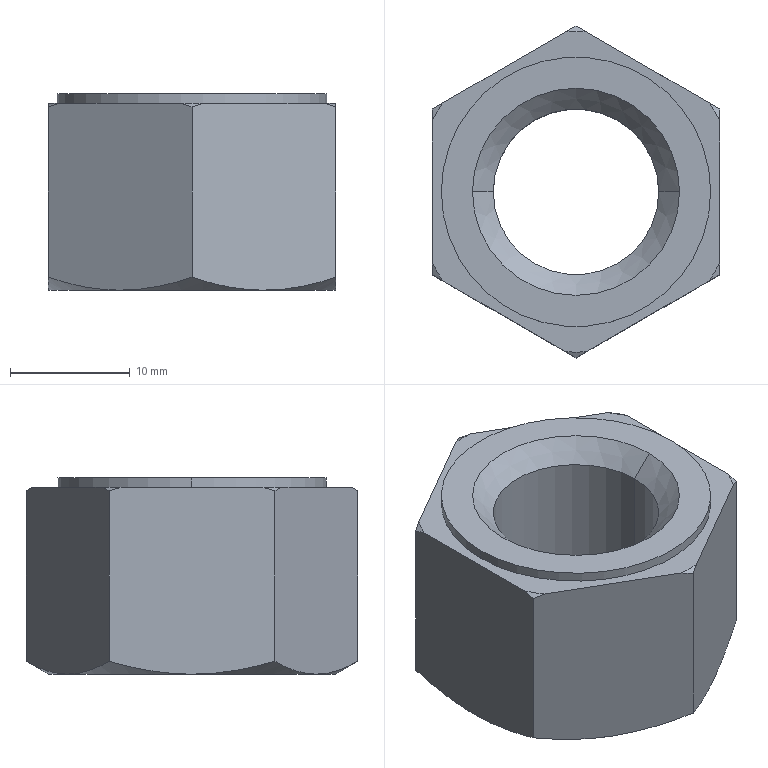Part | SolidWorks | features BaseBody 1 | 1 solid | 29 faces | box 24 x 27.713 x 16.4 mm | volume 5478 mm3 | cone 16 | plane 9 | cylinder 4 | commonest cylinder face diameters 13.835 x2 22.5 x2
STEP:
#1=CARTESIAN_POINT('',(11.25,0.,15.6));
#2=VERTEX_POINT('',#1);
#3=CARTESIAN_POINT('',(-11.25,0.,15.6));
#4=VERTEX_POINT('',#3);
#5=CARTESIAN_POINT('',(0.,0.,15.6));
#6=DIRECTION('',(0.,0.,1.));
#7=DIRECTION('',(1.,0.,0.));
#8=AXIS2_PLACEMENT_3D('',#5,#6,#7);
#9=CIRCLE('',#8,11.25);
#10=EDGE_CURVE('',#2,#4,#9,.T.);
#11=ORIENTED_EDGE('',*,*,#10,.T.);
#12=CARTESIAN_POINT('',(-11.25,0.,16.4));
#13=VERTEX_POINT('',#12);
#14=CARTESIAN_POINT('',(-11.25,0.,15.6));
#15=DIRECTION('',(0.,0.,1.));
#16=VECTOR('',#15,1000.);
#17=LINE('',#14,#16);
#18=EDGE_CURVE('',#4,#13,#17,.T.);
#19=ORIENTED_EDGE('',*,*,#18,.T.);
#20=CARTESIAN_POINT('',(11.25,0.,16.4));
#21=VERTEX_POINT('',#20);
#22=CARTESIAN_POINT('',(0.,0.,16.4));
#23=DIRECTION('',(0.,0.,1.));
#24=DIRECTION('',(1.,0.,0.));
#25=AXIS2_PLACEMENT_3D('',#22,#23,#24);
#26=CIRCLE('',#25,11.25);
#27=EDGE_CURVE('',#21,#13,#26,.T.);
#28=ORIENTED_EDGE('',*,*,#27,.F.);
#29=CARTESIAN_POINT('',(11.25,0.,15.6));
#30=DIRECTION('',(0.,0.,1.));
#31=VECTOR('',#30,1000.);
#32=LINE('',#29,#31);
#33=EDGE_CURVE('',#2,#21,#32,.T.);
#34=ORIENTED_EDGE('',*,*,#33,.F.);
#35=EDGE_LOOP('',(#11,#19,#28,#34));
#36=FACE_OUTER_BOUND('',#35,.T.);
#37=CARTESIAN_POINT('',(0.,0.,15.6));
#38=DIRECTION('',(0.,0.,1.));
#39=DIRECTION('',(1.,0.,0.));
#40=AXIS2_PLACEMENT_3D('',#37,#38,#39);
#41=CYLINDRICAL_SURFACE('',#40,11.25);
#42=ADVANCED_FACE('',(#36),#41,.T.);
#43=CARTESIAN_POINT('',(-6.918,0.,14.668));
#44=VERTEX_POINT('',#43);
#45=CARTESIAN_POINT('',(6.918,0.,14.668));
#46=VERTEX_POINT('',#45);
#47=CARTESIAN_POINT('',(0.,0.,14.668));
#48=DIRECTION('',(0.,0.,1.));
#49=DIRECTION('',(1.,0.,0.));
#50=AXIS2_PLACEMENT_3D('',#47,#48,#49);
#51=CIRCLE('',#50,6.918);
#52=EDGE_CURVE('',#44,#46,#51,.T.);
#53=ORIENTED_EDGE('',*,*,#52,.F.);
#54=CARTESIAN_POINT('',(-8.65,0.,16.4));
#55=VERTEX_POINT('',#54);
#56=CARTESIAN_POINT('',(-6.918,0.,14.668));
#57=DIRECTION('',(-0.7071,0.,0.7071));
#58=VECTOR('',#57,1000.);
#59=LINE('',#56,#58);
#60=EDGE_CURVE('',#44,#55,#59,.T.);
#61=ORIENTED_EDGE('',*,*,#60,.T.);
#62=CARTESIAN_POINT('',(8.65,0.,16.4));
#63=VERTEX_POINT('',#62);
#64=CARTESIAN_POINT('',(0.,0.,16.4));
#65=DIRECTION('',(0.,0.,-1.));
#66=DIRECTION('',(1.,0.,0.));
#67=AXIS2_PLACEMENT_3D('',#64,#65,#66);
#68=CIRCLE('',#67,8.65);
#69=EDGE_CURVE('',#63,#55,#68,.T.);
#70=ORIENTED_EDGE('',*,*,#69,.F.);
#71=CARTESIAN_POINT('',(6.918,0.,14.668));
#72=DIRECTION('',(0.7071,0.,0.7071));
#73=VECTOR('',#72,1000.);
#74=LINE('',#71,#73);
#75=EDGE_CURVE('',#46,#63,#74,.T.);
#76=ORIENTED_EDGE('',*,*,#75,.F.);
#77=EDGE_LOOP('',(#53,#61,#70,#76));
#78=FACE_OUTER_BOUND('',#77,.T.);
#79=CARTESIAN_POINT('',(0.,0.,14.668));
#80=DIRECTION('',(0.,0.,1.));
#81=DIRECTION('',(1.,0.,0.));
#82=AXIS2_PLACEMENT_3D('',#79,#80,#81);
#83=CONICAL_SURFACE('',#82,6.918,0.7854);
#84=ADVANCED_FACE('',(#78),#83,.F.);
#85=CARTESIAN_POINT('',(6.918,0.,1.733));
#86=VERTEX_POINT('',#85);
#87=CARTESIAN_POINT('',(-6.918,0.,1.733));
#88=VERTEX_POINT('',#87);
#89=CARTESIAN_POINT('',(0.,0.,1.733));
#90=DIRECTION('',(0.,0.,-1.));
#91=DIRECTION('',(1.,0.,0.));
#92=AXIS2_PLACEMENT_3D('',#89,#90,#91);
#93=CIRCLE('',#92,6.918);
#94=EDGE_CURVE('',#86,#88,#93,.T.);
#95=ORIENTED_EDGE('',*,*,#94,.F.);
#96=CARTESIAN_POINT('',(8.65,0.,0.));
#97=VERTEX_POINT('',#96);
#98=CARTESIAN_POINT('',(8.65,0.,0.));
#99=DIRECTION('',(0.7071,0.,-0.7071));
#100=VECTOR('',#99,1000.);
#101=LINE('',#98,#100);
#102=EDGE_CURVE('',#86,#97,#101,.T.);
#103=ORIENTED_EDGE('',*,*,#102,.T.);
#104=CARTESIAN_POINT('',(-8.65,0.,0.));
#105=VERTEX_POINT('',#104);
#106=CARTESIAN_POINT('',(0.,0.,0.));
#107=DIRECTION('',(0.,0.,1.));
#108=DIRECTION('',(1.,0.,0.));
#109=AXIS2_PLACEMENT_3D('',#106,#107,#108);
#110=CIRCLE('',#109,8.65);
#111=EDGE_CURVE('',#105,#97,#110,.T.);
#112=ORIENTED_EDGE('',*,*,#111,.F.);
#113=CARTESIAN_POINT('',(-8.65,0.,0.));
#114=DIRECTION('',(-0.7071,0.,-0.7071));
#115=VECTOR('',#114,1000.);
#116=LINE('',#113,#115);
#117=EDGE_CURVE('',#88,#105,#116,.T.);
#118=ORIENTED_EDGE('',*,*,#117,.F.);
#119=EDGE_LOOP('',(#95,#103,#112,#118));
#120=FACE_OUTER_BOUND('',#119,.T.);
#121=CARTESIAN_POINT('',(0.,0.,0.));
#122=DIRECTION('',(0.,0.,-1.));
#123=DIRECTION('',(-1.,0.,0.));
#124=AXIS2_PLACEMENT_3D('',#121,#122,#123);
#125=CONICAL_SURFACE('',#124,8.65,0.7854);
#126=ADVANCED_FACE('',(#120),#125,.F.);
#127=ORIENTED_EDGE('',*,*,#52,.T.);
#128=CARTESIAN_POINT('',(6.918,0.,16.4));
#129=DIRECTION('',(0.,0.,-1.));
#130=VECTOR('',#129,1000.);
#131=LINE('',#128,#130);
#132=EDGE_CURVE('',#46,#86,#131,.T.);
#133=ORIENTED_EDGE('',*,*,#132,.T.);
#134=ORIENTED_EDGE('',*,*,#94,.T.);
#135=CARTESIAN_POINT('',(-6.918,0.,16.4));
#136=DIRECTION('',(0.,0.,-1.));
#137=VECTOR('',#136,1000.);
#138=LINE('',#135,#137);
#139=EDGE_CURVE('',#44,#88,#138,.T.);
#140=ORIENTED_EDGE('',*,*,#139,.F.);
#141=EDGE_LOOP('',(#127,#133,#134,#140));
#142=FACE_OUTER_BOUND('',#141,.T.);
#143=CARTESIAN_POINT('',(0.,0.,16.4));
#144=DIRECTION('',(0.,0.,-1.));
#145=DIRECTION('',(-1.,0.,0.));
#146=AXIS2_PLACEMENT_3D('',#143,#144,#145);
#147=CYLINDRICAL_SURFACE('',#146,6.918);
#148=ADVANCED_FACE('',(#142),#147,.F.);
#149=CARTESIAN_POINT('',(11.136,7.427,15.6));
#150=VERTEX_POINT('',#149);
#151=CARTESIAN_POINT('',(0.8637,13.358,15.6));
#152=VERTEX_POINT('',#151);
#153=CARTESIAN_POINT('',(12.,6.928,15.6));
#154=DIRECTION('',(-0.866,0.5,0.));
#155=VECTOR('',#154,1000.);
#156=LINE('',#153,#155);
#157=EDGE_CURVE('',#150,#152,#156,.T.);
#158=ORIENTED_EDGE('',*,*,#157,.F.);
#159=CARTESIAN_POINT('',(12.,6.928,15.328));
#160=VERTEX_POINT('',#159);
#161=CARTESIAN_POINT('',(12.,6.928,15.328));
#162=CARTESIAN_POINT('',(11.713,7.094,15.424));
#163=CARTESIAN_POINT('',(11.425,7.26,15.515));
#164=CARTESIAN_POINT('',(11.136,7.427,15.6));
#165=B_SPLINE_CURVE_WITH_KNOTS('',3,(#161,#162,#163,#164),.UNSPECIFIED.,.F.,.F.,(4,4),(0.000000238,0.001026),.UNSPECIFIED.);
#166=EDGE_CURVE('',#160,#150,#165,.T.);
#167=ORIENTED_EDGE('',*,*,#166,.F.);
#168=CARTESIAN_POINT('',(12.,6.928,1.072));
#169=VERTEX_POINT('',#168);
#170=CARTESIAN_POINT('',(12.,6.928,16.4));
#171=DIRECTION('',(0.,0.,-1.));
#172=VECTOR('',#171,1000.);
#173=LINE('',#170,#172);
#174=EDGE_CURVE('',#160,#169,#173,.T.);
#175=ORIENTED_EDGE('',*,*,#174,.T.);
#176=CARTESIAN_POINT('',(6.,10.392,0.));
#177=VERTEX_POINT('',#176);
#178=CARTESIAN_POINT('',(6.,10.392,0.));
#179=CARTESIAN_POINT('',(6.509,10.098,0.));
#180=CARTESIAN_POINT('',(7.021,9.803,0.02533));
#181=CARTESIAN_POINT('',(8.033,9.219,0.1234));
#182=CARTESIAN_POINT('',(8.535,8.929,0.196));
#183=CARTESIAN_POINT('',(10.034,8.063,0.476));
#184=CARTESIAN_POINT('',(11.021,7.493,0.7454));
#185=CARTESIAN_POINT('',(12.,6.928,1.072));
#186=B_SPLINE_CURVE_WITH_KNOTS('',3,(#178,#179,#180,#181,#182,#183,#184,#185),.UNSPECIFIED.,.F.,.F.,(4,2,2,4),(0.00701,0.008756,0.0105,0.01399),.UNSPECIFIED.);
#187=EDGE_CURVE('',#177,#169,#186,.T.);
#188=ORIENTED_EDGE('',*,*,#187,.F.);
#189=CARTESIAN_POINT('',(0.,13.856,1.072));
#190=VERTEX_POINT('',#189);
#191=CARTESIAN_POINT('',(0.,13.856,1.072));
#192=CARTESIAN_POINT('',(0.9815,13.29,0.7446));
#193=CARTESIAN_POINT('',(1.97,12.719,0.4751));
#194=CARTESIAN_POINT('',(3.968,11.565,0.1021));
#195=CARTESIAN_POINT('',(4.978,10.982,0.));
#196=CARTESIAN_POINT('',(6.,10.392,0.));
#197=B_SPLINE_CURVE_WITH_KNOTS('',3,(#191,#192,#193,#194,#195,#196),.UNSPECIFIED.,.F.,.F.,(4,2,4),(0.000000238,0.003505,0.00701),.UNSPECIFIED.);
#198=EDGE_CURVE('',#190,#177,#197,.T.);
#199=ORIENTED_EDGE('',*,*,#198,.F.);
#200=CARTESIAN_POINT('',(0.,13.856,15.328));
#201=VERTEX_POINT('',#200);
#202=CARTESIAN_POINT('',(0.,13.856,16.4));
#203=DIRECTION('',(0.,0.,-1.));
#204=VECTOR('',#203,1000.);
#205=LINE('',#202,#204);
#206=EDGE_CURVE('',#201,#190,#205,.T.);
#207=ORIENTED_EDGE('',*,*,#206,.F.);
#208=CARTESIAN_POINT('',(0.8637,13.358,15.6));
#209=CARTESIAN_POINT('',(0.575,13.524,15.515));
#210=CARTESIAN_POINT('',(0.2872,13.691,15.424));
#211=CARTESIAN_POINT('',(0.,13.856,15.328));
#212=B_SPLINE_CURVE_WITH_KNOTS('',3,(#208,#209,#210,#211),.UNSPECIFIED.,.F.,.F.,(4,4),(0.01297,0.01399),.UNSPECIFIED.);
#213=EDGE_CURVE('',#152,#201,#212,.T.);
#214=ORIENTED_EDGE('',*,*,#213,.F.);
#215=EDGE_LOOP('',(#158,#167,#175,#188,#199,#207,#214));
#216=FACE_OUTER_BOUND('',#215,.T.);
#217=CARTESIAN_POINT('',(12.,6.928,16.4));
#218=DIRECTION('',(-0.5,-0.866,0.));
#219=DIRECTION('',(0.866,-0.5,0.));
#220=AXIS2_PLACEMENT_3D('',#217,#218,#219);
#221=PLANE('',#220);
#222=ADVANCED_FACE('',(#216),#221,.F.);
#223=CARTESIAN_POINT('',(-0.8637,13.358,15.6));
#224=VERTEX_POINT('',#223);
#225=CARTESIAN_POINT('',(-11.136,7.427,15.6));
#226=VERTEX_POINT('',#225);
#227=CARTESIAN_POINT('',(0.,13.856,15.6));
#228=DIRECTION('',(-0.866,-0.5,0.));
#229=VECTOR('',#228,1000.);
#230=LINE('',#227,#229);
#231=EDGE_CURVE('',#224,#226,#230,.T.);
#232=ORIENTED_EDGE('',*,*,#231,.F.);
#233=CARTESIAN_POINT('',(0.,13.856,15.328));
#234=CARTESIAN_POINT('',(-0.2873,13.691,15.424));
#235=CARTESIAN_POINT('',(-0.5751,13.524,15.515));
#236=CARTESIAN_POINT('',(-0.8637,13.358,15.6));
#237=B_SPLINE_CURVE_WITH_KNOTS('',3,(#233,#234,#235,#236),.UNSPECIFIED.,.F.,.F.,(4,4),(0.000000238,0.001026),.UNSPECIFIED.);
#238=EDGE_CURVE('',#201,#224,#237,.T.);
#239=ORIENTED_EDGE('',*,*,#238,.F.);
#240=ORIENTED_EDGE('',*,*,#206,.T.);
#241=CARTESIAN_POINT('',(-6.,10.392,0.));
#242=VERTEX_POINT('',#241);
#243=CARTESIAN_POINT('',(-6.,10.392,0.));
#244=CARTESIAN_POINT('',(-5.491,10.686,0.));
#245=CARTESIAN_POINT('',(-4.979,10.982,0.02533));
#246=CARTESIAN_POINT('',(-3.967,11.566,0.1234));
#247=CARTESIAN_POINT('',(-3.465,11.856,0.196));
#248=CARTESIAN_POINT('',(-1.966,12.721,0.476));
#249=CARTESIAN_POINT('',(-0.9791,13.291,0.7454));
#250=CARTESIAN_POINT('',(0.,13.856,1.072));
#251=B_SPLINE_CURVE_WITH_KNOTS('',3,(#243,#244,#245,#246,#247,#248,#249,#250),.UNSPECIFIED.,.F.,.F.,(4,2,2,4),(0.00701,0.008756,0.0105,0.01399),.UNSPECIFIED.);
#252=EDGE_CURVE('',#242,#190,#251,.T.);
#253=ORIENTED_EDGE('',*,*,#252,.F.);
#254=CARTESIAN_POINT('',(-12.,6.928,1.072));
#255=VERTEX_POINT('',#254);
#256=CARTESIAN_POINT('',(-12.,6.928,1.072));
#257=CARTESIAN_POINT('',(-11.018,7.495,0.7446));
#258=CARTESIAN_POINT('',(-10.03,8.066,0.4751));
#259=CARTESIAN_POINT('',(-8.032,9.219,0.1021));
#260=CARTESIAN_POINT('',(-7.022,9.802,0.));
#261=CARTESIAN_POINT('',(-6.,10.392,0.));
#262=B_SPLINE_CURVE_WITH_KNOTS('',3,(#256,#257,#258,#259,#260,#261),.UNSPECIFIED.,.F.,.F.,(4,2,4),(0.000000238,0.003505,0.00701),.UNSPECIFIED.);
#263=EDGE_CURVE('',#255,#242,#262,.T.);
#264=ORIENTED_EDGE('',*,*,#263,.F.);
#265=CARTESIAN_POINT('',(-12.,6.928,15.328));
#266=VERTEX_POINT('',#265);
#267=CARTESIAN_POINT('',(-12.,6.928,16.4));
#268=DIRECTION('',(0.,0.,-1.));
#269=VECTOR('',#268,1000.);
#270=LINE('',#267,#269);
#271=EDGE_CURVE('',#266,#255,#270,.T.);
#272=ORIENTED_EDGE('',*,*,#271,.F.);
#273=CARTESIAN_POINT('',(-11.136,7.427,15.6));
#274=CARTESIAN_POINT('',(-11.425,7.26,15.515));
#275=CARTESIAN_POINT('',(-11.713,7.094,15.424));
#276=CARTESIAN_POINT('',(-12.,6.928,15.328));
#277=B_SPLINE_CURVE_WITH_KNOTS('',3,(#273,#274,#275,#276),.UNSPECIFIED.,.F.,.F.,(4,4),(0.01297,0.01399),.UNSPECIFIED.);
#278=EDGE_CURVE('',#226,#266,#277,.T.);
#279=ORIENTED_EDGE('',*,*,#278,.F.);
#280=EDGE_LOOP('',(#232,#239,#240,#253,#264,#272,#279));
#281=FACE_OUTER_BOUND('',#280,.T.);
#282=CARTESIAN_POINT('',(0.,13.856,16.4));
#283=DIRECTION('',(0.5,-0.866,0.));
#284=DIRECTION('',(0.866,0.5,0.));
#285=AXIS2_PLACEMENT_3D('',#282,#283,#284);
#286=PLANE('',#285);
#287=ADVANCED_FACE('',(#281),#286,.F.);
#288=CARTESIAN_POINT('',(-12.,5.931,15.6));
#289=VERTEX_POINT('',#288);
#290=CARTESIAN_POINT('',(-12.,-5.931,15.6));
#291=VERTEX_POINT('',#290);
#292=CARTESIAN_POINT('',(-12.,6.928,15.6));
#293=DIRECTION('',(0.,-1.,0.));
#294=VECTOR('',#293,1000.);
#295=LINE('',#292,#294);
#296=EDGE_CURVE('',#289,#291,#295,.T.);
#297=ORIENTED_EDGE('',*,*,#296,.F.);
#298=CARTESIAN_POINT('',(-12.,6.928,15.328));
#299=CARTESIAN_POINT('',(-12.,6.597,15.424));
#300=CARTESIAN_POINT('',(-12.,6.265,15.515));
#301=CARTESIAN_POINT('',(-12.,5.931,15.6));
#302=B_SPLINE_CURVE_WITH_KNOTS('',3,(#298,#299,#300,#301),.UNSPECIFIED.,.F.,.F.,(4,4),(0.04083,0.04186),.UNSPECIFIED.);
#303=EDGE_CURVE('',#266,#289,#302,.T.);
#304=ORIENTED_EDGE('',*,*,#303,.F.);
#305=ORIENTED_EDGE('',*,*,#271,.T.);
#306=CARTESIAN_POINT('',(-12.,0.,0.));
#307=VERTEX_POINT('',#306);
#308=CARTESIAN_POINT('',(-12.,0.,0.));
#309=CARTESIAN_POINT('',(-12.,0.5864,0.));
#310=CARTESIAN_POINT('',(-12.,1.176,0.02502));
#311=CARTESIAN_POINT('',(-12.,2.355,0.1241));
#312=CARTESIAN_POINT('',(-12.,2.939,0.1975));
#313=CARTESIAN_POINT('',(-12.,4.673,0.4791));
#314=CARTESIAN_POINT('',(-12.,5.808,0.7483));
#315=CARTESIAN_POINT('',(-12.,6.928,1.072));
#316=B_SPLINE_CURVE_WITH_KNOTS('',3,(#308,#309,#310,#311,#312,#313,#314,#315),.UNSPECIFIED.,.F.,.F.,(4,2,2,4),(0.01976,0.02151,0.02327,0.02678),.UNSPECIFIED.);
#317=EDGE_CURVE('',#307,#255,#316,.T.);
#318=ORIENTED_EDGE('',*,*,#317,.F.);
#319=CARTESIAN_POINT('',(-12.,-6.928,1.072));
#320=VERTEX_POINT('',#319);
#321=CARTESIAN_POINT('',(-12.,-6.928,1.072));
#322=CARTESIAN_POINT('',(-12.,-5.8,0.7462));
#323=CARTESIAN_POINT('',(-12.,-4.647,0.4736));
#324=CARTESIAN_POINT('',(-12.,-2.335,0.1008));
#325=CARTESIAN_POINT('',(-12.,-1.172,0.));
#326=CARTESIAN_POINT('',(-12.,0.,0.));
#327=B_SPLINE_CURVE_WITH_KNOTS('',3,(#321,#322,#323,#324,#325,#326),.UNSPECIFIED.,.F.,.F.,(4,2,4),(0.01275,0.01625,0.01976),.UNSPECIFIED.);
#328=EDGE_CURVE('',#320,#307,#327,.T.);
#329=ORIENTED_EDGE('',*,*,#328,.F.);
#330=CARTESIAN_POINT('',(-12.,-6.928,15.328));
#331=VERTEX_POINT('',#330);
#332=CARTESIAN_POINT('',(-12.,-6.928,16.4));
#333=DIRECTION('',(0.,0.,-1.));
#334=VECTOR('',#333,1000.);
#335=LINE('',#332,#334);
#336=EDGE_CURVE('',#331,#320,#335,.T.);
#337=ORIENTED_EDGE('',*,*,#336,.F.);
#338=CARTESIAN_POINT('',(-12.,-5.931,15.6));
#339=CARTESIAN_POINT('',(-12.,-6.265,15.514));
#340=CARTESIAN_POINT('',(-12.,-6.598,15.424));
#341=CARTESIAN_POINT('',(-12.,-6.928,15.328));
#342=B_SPLINE_CURVE_WITH_KNOTS('',3,(#338,#339,#340,#341),.UNSPECIFIED.,.F.,.F.,(4,4),(0.05382,0.05485),.UNSPECIFIED.);
#343=EDGE_CURVE('',#291,#331,#342,.T.);
#344=ORIENTED_EDGE('',*,*,#343,.F.);
#345=EDGE_LOOP('',(#297,#304,#305,#318,#329,#337,#344));
#346=FACE_OUTER_BOUND('',#345,.T.);
#347=CARTESIAN_POINT('',(-12.,6.928,16.4));
#348=DIRECTION('',(1.,0.,0.));
#349=DIRECTION('',(0.,1.,0.));
#350=AXIS2_PLACEMENT_3D('',#347,#348,#349);
#351=PLANE('',#350);
#352=ADVANCED_FACE('',(#346),#351,.F.);
#353=CARTESIAN_POINT('',(-11.136,-7.427,15.6));
#354=VERTEX_POINT('',#353);
#355=CARTESIAN_POINT('',(-0.8637,-13.358,15.6));
#356=VERTEX_POINT('',#355);
#357=CARTESIAN_POINT('',(-12.,-6.928,15.6));
#358=DIRECTION('',(0.866,-0.5,0.));
#359=VECTOR('',#358,1000.);
#360=LINE('',#357,#359);
#361=EDGE_CURVE('',#354,#356,#360,.T.);
#362=ORIENTED_EDGE('',*,*,#361,.F.);
#363=CARTESIAN_POINT('',(-12.,-6.928,15.328));
#364=CARTESIAN_POINT('',(-11.713,-7.094,15.424));
#365=CARTESIAN_POINT('',(-11.425,-7.26,15.515));
#366=CARTESIAN_POINT('',(-11.136,-7.427,15.6));
#367=B_SPLINE_CURVE_WITH_KNOTS('',3,(#363,#364,#365,#366),.UNSPECIFIED.,.F.,.F.,(4,4),(0.000000238,0.001026),.UNSPECIFIED.);
#368=EDGE_CURVE('',#331,#354,#367,.T.);
#369=ORIENTED_EDGE('',*,*,#368,.F.);
#370=ORIENTED_EDGE('',*,*,#336,.T.);
#371=CARTESIAN_POINT('',(-6.,-10.392,0.));
#372=VERTEX_POINT('',#371);
#373=CARTESIAN_POINT('',(-6.,-10.392,0.));
#374=CARTESIAN_POINT('',(-6.509,-10.098,0.));
#375=CARTESIAN_POINT('',(-7.021,-9.803,0.02533));
#376=CARTESIAN_POINT('',(-8.033,-9.219,0.1234));
#377=CARTESIAN_POINT('',(-8.535,-8.929,0.196));
#378=CARTESIAN_POINT('',(-10.034,-8.063,0.476));
#379=CARTESIAN_POINT('',(-11.021,-7.493,0.7454));
#380=CARTESIAN_POINT('',(-12.,-6.928,1.072));
#381=B_SPLINE_CURVE_WITH_KNOTS('',3,(#373,#374,#375,#376,#377,#378,#379,#380),.UNSPECIFIED.,.F.,.F.,(4,2,2,4),(0.00701,0.008756,0.0105,0.01399),.UNSPECIFIED.);
#382=EDGE_CURVE('',#372,#320,#381,.T.);
#383=ORIENTED_EDGE('',*,*,#382,.F.);
#384=CARTESIAN_POINT('',(0.,-13.856,1.072));
#385=VERTEX_POINT('',#384);
#386=CARTESIAN_POINT('',(0.,-13.856,1.072));
#387=CARTESIAN_POINT('',(-0.9815,-13.29,0.7446));
#388=CARTESIAN_POINT('',(-1.97,-12.719,0.4751));
#389=CARTESIAN_POINT('',(-3.968,-11.565,0.1021));
#390=CARTESIAN_POINT('',(-4.978,-10.982,0.));
#391=CARTESIAN_POINT('',(-6.,-10.392,0.));
#392=B_SPLINE_CURVE_WITH_KNOTS('',3,(#386,#387,#388,#389,#390,#391),.UNSPECIFIED.,.F.,.F.,(4,2,4),(0.000000238,0.003505,0.00701),.UNSPECIFIED.);
#393=EDGE_CURVE('',#385,#372,#392,.T.);
#394=ORIENTED_EDGE('',*,*,#393,.F.);
#395=CARTESIAN_POINT('',(0.,-13.856,15.328));
#396=VERTEX_POINT('',#395);
#397=CARTESIAN_POINT('',(0.,-13.856,16.4));
#398=DIRECTION('',(0.,0.,-1.));
#399=VECTOR('',#398,1000.);
#400=LINE('',#397,#399);
#401=EDGE_CURVE('',#396,#385,#400,.T.);
#402=ORIENTED_EDGE('',*,*,#401,.F.);
#403=CARTESIAN_POINT('',(-0.8637,-13.358,15.6));
#404=CARTESIAN_POINT('',(-0.575,-13.524,15.515));
#405=CARTESIAN_POINT('',(-0.2872,-13.691,15.424));
#406=CARTESIAN_POINT('',(0.,-13.856,15.328));
#407=B_SPLINE_CURVE_WITH_KNOTS('',3,(#403,#404,#405,#406),.UNSPECIFIED.,.F.,.F.,(4,4),(0.01297,0.01399),.UNSPECIFIED.);
#408=EDGE_CURVE('',#356,#396,#407,.T.);
#409=ORIENTED_EDGE('',*,*,#408,.F.);
#410=EDGE_LOOP('',(#362,#369,#370,#383,#394,#402,#409));
#411=FACE_OUTER_BOUND('',#410,.T.);
#412=CARTESIAN_POINT('',(-12.,-6.928,16.4));
#413=DIRECTION('',(0.5,0.866,0.));
#414=DIRECTION('',(-0.866,0.5,0.));
#415=AXIS2_PLACEMENT_3D('',#412,#413,#414);
#416=PLANE('',#415);
#417=ADVANCED_FACE('',(#411),#416,.F.);
#418=CARTESIAN_POINT('',(0.8637,-13.358,15.6));
#419=VERTEX_POINT('',#418);
#420=CARTESIAN_POINT('',(11.136,-7.427,15.6));
#421=VERTEX_POINT('',#420);
#422=CARTESIAN_POINT('',(0.,-13.856,15.6));
#423=DIRECTION('',(0.866,0.5,0.));
#424=VECTOR('',#423,1000.);
#425=LINE('',#422,#424);
#426=EDGE_CURVE('',#419,#421,#425,.T.);
#427=ORIENTED_EDGE('',*,*,#426,.F.);
#428=CARTESIAN_POINT('',(0.,-13.856,15.328));
#429=CARTESIAN_POINT('',(0.2873,-13.691,15.424));
#430=CARTESIAN_POINT('',(0.5751,-13.524,15.515));
#431=CARTESIAN_POINT('',(0.8637,-13.358,15.6));
#432=B_SPLINE_CURVE_WITH_KNOTS('',3,(#428,#429,#430,#431),.UNSPECIFIED.,.F.,.F.,(4,4),(0.000000238,0.001026),.UNSPECIFIED.);
#433=EDGE_CURVE('',#396,#419,#432,.T.);
#434=ORIENTED_EDGE('',*,*,#433,.F.);
#435=ORIENTED_EDGE('',*,*,#401,.T.);
#436=CARTESIAN_POINT('',(6.,-10.392,0.));
#437=VERTEX_POINT('',#436);
#438=CARTESIAN_POINT('',(6.,-10.392,0.));
#439=CARTESIAN_POINT('',(5.491,-10.686,0.));
#440=CARTESIAN_POINT('',(4.979,-10.982,0.02533));
#441=CARTESIAN_POINT('',(3.967,-11.566,0.1234));
#442=CARTESIAN_POINT('',(3.465,-11.856,0.196));
#443=CARTESIAN_POINT('',(1.966,-12.721,0.476));
#444=CARTESIAN_POINT('',(0.9791,-13.291,0.7454));
#445=CARTESIAN_POINT('',(0.,-13.856,1.072));
#446=B_SPLINE_CURVE_WITH_KNOTS('',3,(#438,#439,#440,#441,#442,#443,#444,#445),.UNSPECIFIED.,.F.,.F.,(4,2,2,4),(0.00701,0.008756,0.0105,0.01399),.UNSPECIFIED.);
#447=EDGE_CURVE('',#437,#385,#446,.T.);
#448=ORIENTED_EDGE('',*,*,#447,.F.);
#449=CARTESIAN_POINT('',(12.,-6.928,1.072));
#450=VERTEX_POINT('',#449);
#451=CARTESIAN_POINT('',(12.,-6.928,1.072));
#452=CARTESIAN_POINT('',(11.018,-7.495,0.7446));
#453=CARTESIAN_POINT('',(10.03,-8.066,0.4751));
#454=CARTESIAN_POINT('',(8.032,-9.219,0.1021));
#455=CARTESIAN_POINT('',(7.022,-9.802,0.));
#456=CARTESIAN_POINT('',(6.,-10.392,0.));
#457=B_SPLINE_CURVE_WITH_KNOTS('',3,(#451,#452,#453,#454,#455,#456),.UNSPECIFIED.,.F.,.F.,(4,2,4),(0.000000238,0.003505,0.00701),.UNSPECIFIED.);
#458=EDGE_CURVE('',#450,#437,#457,.T.);
#459=ORIENTED_EDGE('',*,*,#458,.F.);
#460=CARTESIAN_POINT('',(12.,-6.928,15.328));
#461=VERTEX_POINT('',#460);
#462=CARTESIAN_POINT('',(12.,-6.928,16.4));
#463=DIRECTION('',(0.,0.,-1.));
#464=VECTOR('',#463,1000.);
#465=LINE('',#462,#464);
#466=EDGE_CURVE('',#461,#450,#465,.T.);
#467=ORIENTED_EDGE('',*,*,#466,.F.);
#468=CARTESIAN_POINT('',(11.136,-7.427,15.6));
#469=CARTESIAN_POINT('',(11.425,-7.26,15.515));
#470=CARTESIAN_POINT('',(11.713,-7.094,15.424));
#471=CARTESIAN_POINT('',(12.,-6.928,15.328));
#472=B_SPLINE_CURVE_WITH_KNOTS('',3,(#468,#469,#470,#471),.UNSPECIFIED.,.F.,.F.,(4,4),(0.01297,0.01399),.UNSPECIFIED.);
#473=EDGE_CURVE('',#421,#461,#472,.T.);
#474=ORIENTED_EDGE('',*,*,#473,.F.);
#475=EDGE_LOOP('',(#427,#434,#435,#448,#459,#467,#474));
#476=FACE_OUTER_BOUND('',#475,.T.);
#477=CARTESIAN_POINT('',(0.,-13.856,16.4));
#478=DIRECTION('',(-0.5,0.866,0.));
#479=DIRECTION('',(-0.866,-0.5,0.));
#480=AXIS2_PLACEMENT_3D('',#477,#478,#479);
#481=PLANE('',#480);
#482=ADVANCED_FACE('',(#476),#481,.F.);
#483=CARTESIAN_POINT('',(12.,-5.931,15.6));
#484=VERTEX_POINT('',#483);
#485=CARTESIAN_POINT('',(12.,5.931,15.6));
#486=VERTEX_POINT('',#485);
#487=CARTESIAN_POINT('',(12.,-6.928,15.6));
#488=DIRECTION('',(0.,1.,0.));
#489=VECTOR('',#488,1000.);
#490=LINE('',#487,#489);
#491=EDGE_CURVE('',#484,#486,#490,.T.);
#492=ORIENTED_EDGE('',*,*,#491,.F.);
#493=CARTESIAN_POINT('',(12.,-6.928,15.328));
#494=CARTESIAN_POINT('',(12.,-6.598,15.424));
#495=CARTESIAN_POINT('',(12.,-6.265,15.514));
#496=CARTESIAN_POINT('',(12.,-5.931,15.6));
#497=B_SPLINE_CURVE_WITH_KNOTS('',3,(#493,#494,#495,#496),.UNSPECIFIED.,.F.,.F.,(4,4),(0.01275,0.01377),.UNSPECIFIED.);
#498=EDGE_CURVE('',#461,#484,#497,.T.);
#499=ORIENTED_EDGE('',*,*,#498,.F.);
#500=ORIENTED_EDGE('',*,*,#466,.T.);
#501=CARTESIAN_POINT('',(12.,0.,0.));
#502=VERTEX_POINT('',#501);
#503=CARTESIAN_POINT('',(12.,0.,0.));
#504=CARTESIAN_POINT('',(12.,-1.172,0.));
#505=CARTESIAN_POINT('',(12.,-2.335,0.1008));
#506=CARTESIAN_POINT('',(12.,-4.647,0.4736));
#507=CARTESIAN_POINT('',(12.,-5.8,0.7462));
#508=CARTESIAN_POINT('',(12.,-6.928,1.072));
#509=B_SPLINE_CURVE_WITH_KNOTS('',3,(#503,#504,#505,#506,#507,#508),.UNSPECIFIED.,.F.,.F.,(4,2,4),(0.04784,0.05135,0.05485),.UNSPECIFIED.);
#510=EDGE_CURVE('',#502,#450,#509,.T.);
#511=ORIENTED_EDGE('',*,*,#510,.F.);
#512=CARTESIAN_POINT('',(12.,6.928,1.072));
#513=CARTESIAN_POINT('',(12.,5.808,0.7483));
#514=CARTESIAN_POINT('',(12.,4.673,0.4791));
#515=CARTESIAN_POINT('',(12.,2.939,0.1975));
#516=CARTESIAN_POINT('',(12.,2.355,0.1241));
#517=CARTESIAN_POINT('',(12.,1.176,0.02502));
#518=CARTESIAN_POINT('',(12.,0.5864,0.));
#519=CARTESIAN_POINT('',(12.,0.,0.));
#520=B_SPLINE_CURVE_WITH_KNOTS('',3,(#512,#513,#514,#515,#516,#517,#518,#519),.UNSPECIFIED.,.F.,.F.,(4,2,2,4),(0.04083,0.04433,0.04609,0.04784),.UNSPECIFIED.);
#521=EDGE_CURVE('',#169,#502,#520,.T.);
#522=ORIENTED_EDGE('',*,*,#521,.F.);
#523=ORIENTED_EDGE('',*,*,#174,.F.);
#524=CARTESIAN_POINT('',(12.,5.931,15.6));
#525=CARTESIAN_POINT('',(12.,6.265,15.515));
#526=CARTESIAN_POINT('',(12.,6.597,15.424));
#527=CARTESIAN_POINT('',(12.,6.928,15.328));
#528=B_SPLINE_CURVE_WITH_KNOTS('',3,(#524,#525,#526,#527),.UNSPECIFIED.,.F.,.F.,(4,4),(0.02574,0.02678),.UNSPECIFIED.);
#529=EDGE_CURVE('',#486,#160,#528,.T.);
#530=ORIENTED_EDGE('',*,*,#529,.F.);
#531=EDGE_LOOP('',(#492,#499,#500,#511,#522,#523,#530));
#532=FACE_OUTER_BOUND('',#531,.T.);
#533=CARTESIAN_POINT('',(12.,-6.928,16.4));
#534=DIRECTION('',(-1.,0.,0.));
#535=DIRECTION('',(0.,-1.,0.));
#536=AXIS2_PLACEMENT_3D('',#533,#534,#535);
#537=PLANE('',#536);
#538=ADVANCED_FACE('',(#532),#537,.F.);
#539=ORIENTED_EDGE('',*,*,#69,.T.);
#540=CARTESIAN_POINT('',(0.,0.,16.4));
#541=DIRECTION('',(0.,0.,-1.));
#542=DIRECTION('',(1.,0.,0.));
#543=AXIS2_PLACEMENT_3D('',#540,#541,#542);
#544=CIRCLE('',#543,8.65);
#545=EDGE_CURVE('',#55,#63,#544,.T.);
#546=ORIENTED_EDGE('',*,*,#545,.T.);
#547=EDGE_LOOP('',(#539,#546));
#548=FACE_BOUND('',#547,.T.);
#549=ORIENTED_EDGE('',*,*,#27,.T.);
#550=CARTESIAN_POINT('',(0.,0.,16.4));
#551=DIRECTION('',(0.,0.,1.));
#552=DIRECTION('',(1.,0.,0.));
#553=AXIS2_PLACEMENT_3D('',#550,#551,#552);
#554=CIRCLE('',#553,11.25);
#555=EDGE_CURVE('',#13,#21,#554,.T.);
#556=ORIENTED_EDGE('',*,*,#555,.T.);
#557=EDGE_LOOP('',(#549,#556));
#558=FACE_OUTER_BOUND('',#557,.T.);
#559=CARTESIAN_POINT('',(-12.,20.785,16.4));
#560=DIRECTION('',(0.,0.,1.));
#561=DIRECTION('',(1.,0.,0.));
#562=AXIS2_PLACEMENT_3D('',#559,#560,#561);
#563=PLANE('',#562);
#564=ADVANCED_FACE('',(#548,#558),#563,.T.);
#565=ORIENTED_EDGE('',*,*,#498,.T.);
#566=CARTESIAN_POINT('',(0.,0.,15.6));
#567=DIRECTION('',(0.,0.,-1.));
#568=DIRECTION('',(1.,0.,0.));
#569=AXIS2_PLACEMENT_3D('',#566,#567,#568);
#570=CIRCLE('',#569,13.386);
#571=EDGE_CURVE('',#484,#421,#570,.T.);
#572=ORIENTED_EDGE('',*,*,#571,.T.);
#573=ORIENTED_EDGE('',*,*,#473,.T.);
#574=EDGE_LOOP('',(#565,#572,#573));
#575=FACE_OUTER_BOUND('',#574,.T.);
#576=CARTESIAN_POINT('',(0.,0.,16.4));
#577=DIRECTION('',(0.,0.,-1.));
#578=DIRECTION('',(1.,0.,0.));
#579=AXIS2_PLACEMENT_3D('',#576,#577,#578);
#580=CONICAL_SURFACE('',#579,12.,1.047);
#581=ADVANCED_FACE('',(#575),#580,.T.);
#582=ORIENTED_EDGE('',*,*,#433,.T.);
#583=CARTESIAN_POINT('',(0.,0.,15.6));
#584=DIRECTION('',(0.,0.,-1.));
#585=DIRECTION('',(1.,0.,0.));
#586=AXIS2_PLACEMENT_3D('',#583,#584,#585);
#587=CIRCLE('',#586,13.386);
#588=EDGE_CURVE('',#419,#356,#587,.T.);
#589=ORIENTED_EDGE('',*,*,#588,.T.);
#590=ORIENTED_EDGE('',*,*,#408,.T.);
#591=EDGE_LOOP('',(#582,#589,#590));
#592=FACE_OUTER_BOUND('',#591,.T.);
#593=CARTESIAN_POINT('',(0.,0.,16.4));
#594=DIRECTION('',(0.,0.,-1.));
#595=DIRECTION('',(1.,0.,0.));
#596=AXIS2_PLACEMENT_3D('',#593,#594,#595);
#597=CONICAL_SURFACE('',#596,12.,1.047);
#598=ADVANCED_FACE('',(#592),#597,.T.);
#599=ORIENTED_EDGE('',*,*,#368,.T.);
#600=CARTESIAN_POINT('',(0.,0.,15.6));
#601=DIRECTION('',(0.,0.,-1.));
#602=DIRECTION('',(1.,0.,0.));
#603=AXIS2_PLACEMENT_3D('',#600,#601,#602);
#604=CIRCLE('',#603,13.386);
#605=EDGE_CURVE('',#354,#291,#604,.T.);
#606=ORIENTED_EDGE('',*,*,#605,.T.);
#607=ORIENTED_EDGE('',*,*,#343,.T.);
#608=EDGE_LOOP('',(#599,#606,#607));
#609=FACE_OUTER_BOUND('',#608,.T.);
#610=CARTESIAN_POINT('',(0.,0.,16.4));
#611=DIRECTION('',(0.,0.,-1.));
#612=DIRECTION('',(1.,0.,0.));
#613=AXIS2_PLACEMENT_3D('',#610,#611,#612);
#614=CONICAL_SURFACE('',#613,12.,1.047);
#615=ADVANCED_FACE('',(#609),#614,.T.);
#616=ORIENTED_EDGE('',*,*,#303,.T.);
#617=CARTESIAN_POINT('',(0.,0.,15.6));
#618=DIRECTION('',(0.,0.,-1.));
#619=DIRECTION('',(1.,0.,0.));
#620=AXIS2_PLACEMENT_3D('',#617,#618,#619);
#621=CIRCLE('',#620,13.386);
#622=EDGE_CURVE('',#289,#226,#621,.T.);
#623=ORIENTED_EDGE('',*,*,#622,.T.);
#624=ORIENTED_EDGE('',*,*,#278,.T.);
#625=EDGE_LOOP('',(#616,#623,#624));
#626=FACE_OUTER_BOUND('',#625,.T.);
#627=CARTESIAN_POINT('',(0.,0.,16.4));
#628=DIRECTION('',(0.,0.,-1.));
#629=DIRECTION('',(1.,0.,0.));
#630=AXIS2_PLACEMENT_3D('',#627,#628,#629);
#631=CONICAL_SURFACE('',#630,12.,1.047);
#632=ADVANCED_FACE('',(#626),#631,.T.);
#633=ORIENTED_EDGE('',*,*,#238,.T.);
#634=CARTESIAN_POINT('',(0.,0.,15.6));
#635=DIRECTION('',(0.,0.,-1.));
#636=DIRECTION('',(1.,0.,0.));
#637=AXIS2_PLACEMENT_3D('',#634,#635,#636);
#638=CIRCLE('',#637,13.386);
#639=EDGE_CURVE('',#224,#152,#638,.T.);
#640=ORIENTED_EDGE('',*,*,#639,.T.);
#641=ORIENTED_EDGE('',*,*,#213,.T.);
#642=EDGE_LOOP('',(#633,#640,#641));
#643=FACE_OUTER_BOUND('',#642,.T.);
#644=CARTESIAN_POINT('',(0.,0.,16.4));
#645=DIRECTION('',(0.,0.,-1.));
#646=DIRECTION('',(1.,0.,0.));
#647=AXIS2_PLACEMENT_3D('',#644,#645,#646);
#648=CONICAL_SURFACE('',#647,12.,1.047);
#649=ADVANCED_FACE('',(#643),#648,.T.);
#650=ORIENTED_EDGE('',*,*,#166,.T.);
#651=CARTESIAN_POINT('',(0.,0.,15.6));
#652=DIRECTION('',(0.,0.,-1.));
#653=DIRECTION('',(1.,0.,0.));
#654=AXIS2_PLACEMENT_3D('',#651,#652,#653);
#655=CIRCLE('',#654,13.386);
#656=EDGE_CURVE('',#150,#486,#655,.T.);
#657=ORIENTED_EDGE('',*,*,#656,.T.);
#658=ORIENTED_EDGE('',*,*,#529,.T.);
#659=EDGE_LOOP('',(#650,#657,#658));
#660=FACE_OUTER_BOUND('',#659,.T.);
#661=CARTESIAN_POINT('',(0.,0.,16.4));
#662=DIRECTION('',(0.,0.,-1.));
#663=DIRECTION('',(1.,0.,0.));
#664=AXIS2_PLACEMENT_3D('',#661,#662,#663);
#665=CONICAL_SURFACE('',#664,12.,1.047);
#666=ADVANCED_FACE('',(#660),#665,.T.);
#667=ORIENTED_EDGE('',*,*,#111,.T.);
#668=CARTESIAN_POINT('',(0.,0.,0.));
#669=DIRECTION('',(0.,0.,1.));
#670=DIRECTION('',(1.,0.,0.));
#671=AXIS2_PLACEMENT_3D('',#668,#669,#670);
#672=CIRCLE('',#671,8.65);
#673=EDGE_CURVE('',#97,#105,#672,.T.);
#674=ORIENTED_EDGE('',*,*,#673,.T.);
#675=EDGE_LOOP('',(#667,#674));
#676=FACE_BOUND('',#675,.T.);
#677=CARTESIAN_POINT('',(0.,0.,0.));
#678=DIRECTION('',(0.,0.,-1.));
#679=DIRECTION('',(-1.,0.,0.));
#680=AXIS2_PLACEMENT_3D('',#677,#678,#679);
#681=CIRCLE('',#680,12.);
#682=EDGE_CURVE('',#177,#502,#681,.T.);
#683=ORIENTED_EDGE('',*,*,#682,.T.);
#684=CARTESIAN_POINT('',(0.,0.,0.));
#685=DIRECTION('',(0.,0.,-1.));
#686=DIRECTION('',(-1.,0.,0.));
#687=AXIS2_PLACEMENT_3D('',#684,#685,#686);
#688=CIRCLE('',#687,12.);
#689=EDGE_CURVE('',#502,#437,#688,.T.);
#690=ORIENTED_EDGE('',*,*,#689,.T.);
#691=CARTESIAN_POINT('',(0.,0.,0.));
#692=DIRECTION('',(0.,0.,-1.));
#693=DIRECTION('',(-1.,0.,0.));
#694=AXIS2_PLACEMENT_3D('',#691,#692,#693);
#695=CIRCLE('',#694,12.);
#696=EDGE_CURVE('',#437,#372,#695,.T.);
#697=ORIENTED_EDGE('',*,*,#696,.T.);
#698=CARTESIAN_POINT('',(0.,0.,0.));
#699=DIRECTION('',(0.,0.,-1.));
#700=DIRECTION('',(-1.,0.,0.));
#701=AXIS2_PLACEMENT_3D('',#698,#699,#700);
#702=CIRCLE('',#701,12.);
#703=EDGE_CURVE('',#372,#307,#702,.T.);
#704=ORIENTED_EDGE('',*,*,#703,.T.);
#705=CARTESIAN_POINT('',(0.,0.,0.));
#706=DIRECTION('',(0.,0.,-1.));
#707=DIRECTION('',(-1.,0.,0.));
#708=AXIS2_PLACEMENT_3D('',#705,#706,#707);
#709=CIRCLE('',#708,12.);
#710=EDGE_CURVE('',#307,#242,#709,.T.);
#711=ORIENTED_EDGE('',*,*,#710,.T.);
#712=CARTESIAN_POINT('',(0.,0.,0.));
#713=DIRECTION('',(0.,0.,-1.));
#714=DIRECTION('',(-1.,0.,0.));
#715=AXIS2_PLACEMENT_3D('',#712,#713,#714);
#716=CIRCLE('',#715,12.);
#717=EDGE_CURVE('',#242,#177,#716,.T.);
#718=ORIENTED_EDGE('',*,*,#717,.T.);
#719=EDGE_LOOP('',(#683,#690,#697,#704,#711,#718));
#720=FACE_OUTER_BOUND('',#719,.T.);
#721=CARTESIAN_POINT('',(-12.,20.785,0.));
#722=DIRECTION('',(0.,0.,1.));
#723=DIRECTION('',(1.,0.,0.));
#724=AXIS2_PLACEMENT_3D('',#721,#722,#723);
#725=PLANE('',#724);
#726=ADVANCED_FACE('',(#676,#720),#725,.F.);
#727=ORIENTED_EDGE('',*,*,#132,.F.);
#728=CARTESIAN_POINT('',(0.,0.,14.668));
#729=DIRECTION('',(0.,0.,1.));
#730=DIRECTION('',(1.,0.,0.));
#731=AXIS2_PLACEMENT_3D('',#728,#729,#730);
#732=CIRCLE('',#731,6.918);
#733=EDGE_CURVE('',#46,#44,#732,.T.);
#734=ORIENTED_EDGE('',*,*,#733,.T.);
#735=ORIENTED_EDGE('',*,*,#139,.T.);
#736=CARTESIAN_POINT('',(0.,0.,1.733));
#737=DIRECTION('',(0.,0.,-1.));
#738=DIRECTION('',(1.,0.,0.));
#739=AXIS2_PLACEMENT_3D('',#736,#737,#738);
#740=CIRCLE('',#739,6.918);
#741=EDGE_CURVE('',#88,#86,#740,.T.);
#742=ORIENTED_EDGE('',*,*,#741,.T.);
#743=EDGE_LOOP('',(#727,#734,#735,#742));
#744=FACE_OUTER_BOUND('',#743,.T.);
#745=CARTESIAN_POINT('',(0.,0.,16.4));
#746=DIRECTION('',(0.,0.,-1.));
#747=DIRECTION('',(-1.,0.,0.));
#748=AXIS2_PLACEMENT_3D('',#745,#746,#747);
#749=CYLINDRICAL_SURFACE('',#748,6.918);
#750=ADVANCED_FACE('',(#744),#749,.F.);
#751=ORIENTED_EDGE('',*,*,#458,.T.);
#752=ORIENTED_EDGE('',*,*,#689,.F.);
#753=ORIENTED_EDGE('',*,*,#510,.T.);
#754=EDGE_LOOP('',(#751,#752,#753));
#755=FACE_OUTER_BOUND('',#754,.T.);
#756=CARTESIAN_POINT('',(0.,0.,0.));
#757=DIRECTION('',(0.,0.,1.));
#758=DIRECTION('',(-1.,0.,0.));
#759=AXIS2_PLACEMENT_3D('',#756,#757,#758);
#760=CONICAL_SURFACE('',#759,12.,1.047);
#761=ADVANCED_FACE('',(#755),#760,.T.);
#762=ORIENTED_EDGE('',*,*,#187,.T.);
#763=ORIENTED_EDGE('',*,*,#521,.T.);
#764=ORIENTED_EDGE('',*,*,#682,.F.);
#765=EDGE_LOOP('',(#762,#763,#764));
#766=FACE_OUTER_BOUND('',#765,.T.);
#767=CARTESIAN_POINT('',(0.,0.,0.));
#768=DIRECTION('',(0.,0.,1.));
#769=DIRECTION('',(-1.,0.,0.));
#770=AXIS2_PLACEMENT_3D('',#767,#768,#769);
#771=CONICAL_SURFACE('',#770,12.,1.047);
#772=ADVANCED_FACE('',(#766),#771,.T.);
#773=ORIENTED_EDGE('',*,*,#393,.T.);
#774=ORIENTED_EDGE('',*,*,#696,.F.);
#775=ORIENTED_EDGE('',*,*,#447,.T.);
#776=EDGE_LOOP('',(#773,#774,#775));
#777=FACE_OUTER_BOUND('',#776,.T.);
#778=CARTESIAN_POINT('',(0.,0.,0.));
#779=DIRECTION('',(0.,0.,1.));
#780=DIRECTION('',(-1.,0.,0.));
#781=AXIS2_PLACEMENT_3D('',#778,#779,#780);
#782=CONICAL_SURFACE('',#781,12.,1.047);
#783=ADVANCED_FACE('',(#777),#782,.T.);
#784=ORIENTED_EDGE('',*,*,#328,.T.);
#785=ORIENTED_EDGE('',*,*,#703,.F.);
#786=ORIENTED_EDGE('',*,*,#382,.T.);
#787=EDGE_LOOP('',(#784,#785,#786));
#788=FACE_OUTER_BOUND('',#787,.T.);
#789=CARTESIAN_POINT('',(0.,0.,0.));
#790=DIRECTION('',(0.,0.,1.));
#791=DIRECTION('',(-1.,0.,0.));
#792=AXIS2_PLACEMENT_3D('',#789,#790,#791);
#793=CONICAL_SURFACE('',#792,12.,1.047);
#794=ADVANCED_FACE('',(#788),#793,.T.);
#795=ORIENTED_EDGE('',*,*,#317,.T.);
#796=ORIENTED_EDGE('',*,*,#263,.T.);
#797=ORIENTED_EDGE('',*,*,#710,.F.);
#798=EDGE_LOOP('',(#795,#796,#797));
#799=FACE_OUTER_BOUND('',#798,.T.);
#800=CARTESIAN_POINT('',(0.,0.,0.));
#801=DIRECTION('',(0.,0.,1.));
#802=DIRECTION('',(-1.,0.,0.));
#803=AXIS2_PLACEMENT_3D('',#800,#801,#802);
#804=CONICAL_SURFACE('',#803,12.,1.047);
#805=ADVANCED_FACE('',(#799),#804,.T.);
#806=ORIENTED_EDGE('',*,*,#252,.T.);
#807=ORIENTED_EDGE('',*,*,#198,.T.);
#808=ORIENTED_EDGE('',*,*,#717,.F.);
#809=EDGE_LOOP('',(#806,#807,#808));
#810=FACE_OUTER_BOUND('',#809,.T.);
#811=CARTESIAN_POINT('',(0.,0.,0.));
#812=DIRECTION('',(0.,0.,1.));
#813=DIRECTION('',(-1.,0.,0.));
#814=AXIS2_PLACEMENT_3D('',#811,#812,#813);
#815=CONICAL_SURFACE('',#814,12.,1.047);
#816=ADVANCED_FACE('',(#810),#815,.T.);
#817=ORIENTED_EDGE('',*,*,#102,.F.);
#818=ORIENTED_EDGE('',*,*,#741,.F.);
#819=ORIENTED_EDGE('',*,*,#117,.T.);
#820=ORIENTED_EDGE('',*,*,#673,.F.);
#821=EDGE_LOOP('',(#817,#818,#819,#820));
#822=FACE_OUTER_BOUND('',#821,.T.);
#823=CARTESIAN_POINT('',(0.,0.,0.));
#824=DIRECTION('',(0.,0.,-1.));
#825=DIRECTION('',(-1.,0.,0.));
#826=AXIS2_PLACEMENT_3D('',#823,#824,#825);
#827=CONICAL_SURFACE('',#826,8.65,0.7854);
#828=ADVANCED_FACE('',(#822),#827,.F.);
#829=ORIENTED_EDGE('',*,*,#60,.F.);
#830=ORIENTED_EDGE('',*,*,#733,.F.);
#831=ORIENTED_EDGE('',*,*,#75,.T.);
#832=ORIENTED_EDGE('',*,*,#545,.F.);
#833=EDGE_LOOP('',(#829,#830,#831,#832));
#834=FACE_OUTER_BOUND('',#833,.T.);
#835=CARTESIAN_POINT('',(0.,0.,14.668));
#836=DIRECTION('',(0.,0.,1.));
#837=DIRECTION('',(1.,0.,0.));
#838=AXIS2_PLACEMENT_3D('',#835,#836,#837);
#839=CONICAL_SURFACE('',#838,6.918,0.7854);
#840=ADVANCED_FACE('',(#834),#839,.F.);
#841=ORIENTED_EDGE('',*,*,#361,.T.);
#842=ORIENTED_EDGE('',*,*,#588,.F.);
#843=ORIENTED_EDGE('',*,*,#426,.T.);
#844=ORIENTED_EDGE('',*,*,#571,.F.);
#845=ORIENTED_EDGE('',*,*,#491,.T.);
#846=ORIENTED_EDGE('',*,*,#656,.F.);
#847=ORIENTED_EDGE('',*,*,#157,.T.);
#848=ORIENTED_EDGE('',*,*,#639,.F.);
#849=ORIENTED_EDGE('',*,*,#231,.T.);
#850=ORIENTED_EDGE('',*,*,#622,.F.);
#851=ORIENTED_EDGE('',*,*,#296,.T.);
#852=ORIENTED_EDGE('',*,*,#605,.F.);
#853=EDGE_LOOP('',(#841,#842,#843,#844,#845,#846,#847,#848,#849,#850,#851,#852));
#854=FACE_OUTER_BOUND('',#853,.T.);
#855=ORIENTED_EDGE('',*,*,#10,.F.);
#856=CARTESIAN_POINT('',(0.,0.,15.6));
#857=DIRECTION('',(0.,0.,1.));
#858=DIRECTION('',(1.,0.,0.));
#859=AXIS2_PLACEMENT_3D('',#856,#857,#858);
#860=CIRCLE('',#859,11.25);
#861=EDGE_CURVE('',#4,#2,#860,.T.);
#862=ORIENTED_EDGE('',*,*,#861,.F.);
#863=EDGE_LOOP('',(#855,#862));
#864=FACE_BOUND('',#863,.T.);
#865=CARTESIAN_POINT('',(0.,0.,15.6));
#866=DIRECTION('',(0.,0.,1.));
#867=DIRECTION('',(1.,0.,0.));
#868=AXIS2_PLACEMENT_3D('',#865,#866,#867);
#869=PLANE('',#868);
#870=ADVANCED_FACE('',(#854,#864),#869,.T.);
#871=ORIENTED_EDGE('',*,*,#18,.F.);
#872=ORIENTED_EDGE('',*,*,#861,.T.);
#873=ORIENTED_EDGE('',*,*,#33,.T.);
#874=ORIENTED_EDGE('',*,*,#555,.F.);
#875=EDGE_LOOP('',(#871,#872,#873,#874));
#876=FACE_OUTER_BOUND('',#875,.T.);
#877=CARTESIAN_POINT('',(0.,0.,15.6));
#878=DIRECTION('',(0.,0.,1.));
#879=DIRECTION('',(1.,0.,0.));
#880=AXIS2_PLACEMENT_3D('',#877,#878,#879);
#881=CYLINDRICAL_SURFACE('',#880,11.25);
#882=ADVANCED_FACE('',(#876),#881,.T.);
#883=CLOSED_SHELL('',(#42,#84,#126,#148,#222,#287,#352,#417,#482,#538,#564,#581,#598,#615,#632,#649,#666,#726,#750,#761,#772,#783,#794,#805,#816,#828,#840,#870,#882));
#884=MANIFOLD_SOLID_BREP('',#883);
#885=CARTESIAN_POINT('',(0.,0.,0.));
#886=DIRECTION('',(0.,0.,1.));
#887=DIRECTION('',(1.,0.,0.));
#888=AXIS2_PLACEMENT_3D('',#885,#886,#887);
#889=(LENGTH_UNIT()NAMED_UNIT(*)SI_UNIT(.MILLI.,.METRE.));
#890=UNCERTAINTY_MEASURE_WITH_UNIT(LENGTH_MEASURE(0.00001),#889,'','');
#891=(NAMED_UNIT(*)PLANE_ANGLE_UNIT()SI_UNIT($,.RADIAN.));
#892=(NAMED_UNIT(*)SI_UNIT($,.STERADIAN.)SOLID_ANGLE_UNIT());
#893=(GEOMETRIC_REPRESENTATION_CONTEXT(3)GLOBAL_UNCERTAINTY_ASSIGNED_CONTEXT((#890))GLOBAL_UNIT_ASSIGNED_CONTEXT((#889,#891,#892))REPRESENTATION_CONTEXT('',''));
#894=ADVANCED_BREP_SHAPE_REPRESENTATION('',(#884,#888),#893);